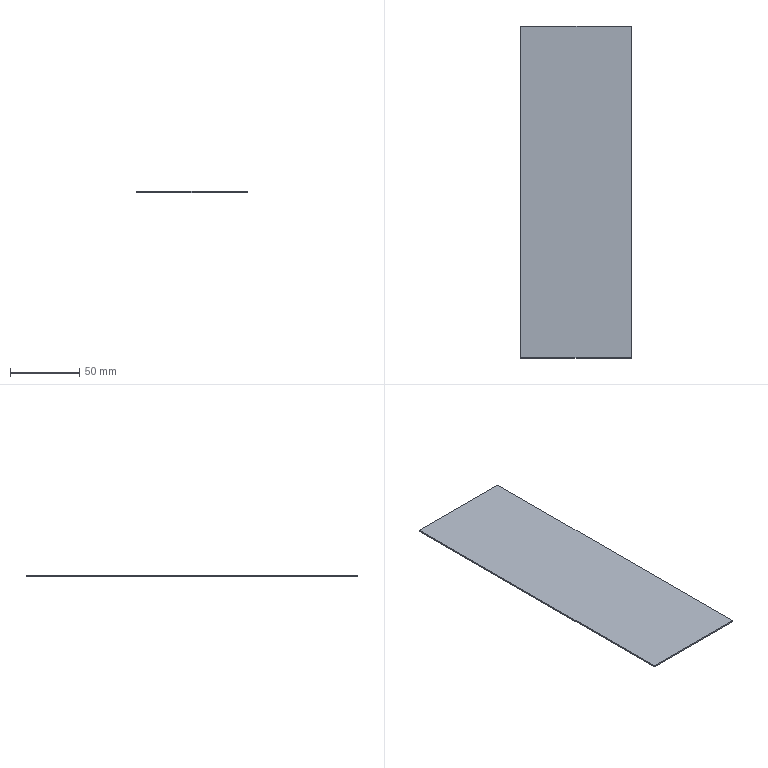Part | SolidWorks | features Extrusion 1 | 1 solid | 6 faces | box 80 x 240 x 1 mm | volume 19200 mm3 | plane 6
STEP:
#1=CARTESIAN_POINT('',(40.,-120.,0.));
#2=VERTEX_POINT('',#1);
#3=CARTESIAN_POINT('',(40.,120.,0.));
#4=VERTEX_POINT('',#3);
#5=CARTESIAN_POINT('',(40.,120.,0.));
#6=DIRECTION('',(0.,1.,0.));
#7=VECTOR('',#6,1000.);
#8=LINE('',#5,#7);
#9=EDGE_CURVE('',#2,#4,#8,.T.);
#10=ORIENTED_EDGE('',*,*,#9,.T.);
#11=CARTESIAN_POINT('',(40.,120.,1.));
#12=VERTEX_POINT('',#11);
#13=CARTESIAN_POINT('',(40.,120.,1.));
#14=DIRECTION('',(0.,0.,-1.));
#15=VECTOR('',#14,1000.);
#16=LINE('',#13,#15);
#17=EDGE_CURVE('',#12,#4,#16,.T.);
#18=ORIENTED_EDGE('',*,*,#17,.F.);
#19=CARTESIAN_POINT('',(40.,-120.,1.));
#20=VERTEX_POINT('',#19);
#21=CARTESIAN_POINT('',(40.,120.,1.));
#22=DIRECTION('',(0.,1.,0.));
#23=VECTOR('',#22,1000.);
#24=LINE('',#21,#23);
#25=EDGE_CURVE('',#20,#12,#24,.T.);
#26=ORIENTED_EDGE('',*,*,#25,.F.);
#27=CARTESIAN_POINT('',(40.,-120.,1.));
#28=DIRECTION('',(0.,0.,-1.));
#29=VECTOR('',#28,1000.);
#30=LINE('',#27,#29);
#31=EDGE_CURVE('',#20,#2,#30,.T.);
#32=ORIENTED_EDGE('',*,*,#31,.T.);
#33=EDGE_LOOP('',(#10,#18,#26,#32));
#34=FACE_OUTER_BOUND('',#33,.T.);
#35=CARTESIAN_POINT('',(40.,120.,1.));
#36=DIRECTION('',(-1.,0.,0.));
#37=DIRECTION('',(0.,-1.,0.));
#38=AXIS2_PLACEMENT_3D('',#35,#36,#37);
#39=PLANE('',#38);
#40=ADVANCED_FACE('',(#34),#39,.F.);
#41=CARTESIAN_POINT('',(-40.,120.,0.));
#42=VERTEX_POINT('',#41);
#43=CARTESIAN_POINT('',(-40.,120.,0.));
#44=DIRECTION('',(-1.,0.,0.));
#45=VECTOR('',#44,1000.);
#46=LINE('',#43,#45);
#47=EDGE_CURVE('',#4,#42,#46,.T.);
#48=ORIENTED_EDGE('',*,*,#47,.T.);
#49=CARTESIAN_POINT('',(-40.,120.,1.));
#50=VERTEX_POINT('',#49);
#51=CARTESIAN_POINT('',(-40.,120.,1.));
#52=DIRECTION('',(0.,0.,-1.));
#53=VECTOR('',#52,1000.);
#54=LINE('',#51,#53);
#55=EDGE_CURVE('',#50,#42,#54,.T.);
#56=ORIENTED_EDGE('',*,*,#55,.F.);
#57=CARTESIAN_POINT('',(-40.,120.,1.));
#58=DIRECTION('',(-1.,0.,0.));
#59=VECTOR('',#58,1000.);
#60=LINE('',#57,#59);
#61=EDGE_CURVE('',#12,#50,#60,.T.);
#62=ORIENTED_EDGE('',*,*,#61,.F.);
#63=ORIENTED_EDGE('',*,*,#17,.T.);
#64=EDGE_LOOP('',(#48,#56,#62,#63));
#65=FACE_OUTER_BOUND('',#64,.T.);
#66=CARTESIAN_POINT('',(-40.,120.,1.));
#67=DIRECTION('',(0.,-1.,0.));
#68=DIRECTION('',(0.,0.,-1.));
#69=AXIS2_PLACEMENT_3D('',#66,#67,#68);
#70=PLANE('',#69);
#71=ADVANCED_FACE('',(#65),#70,.F.);
#72=CARTESIAN_POINT('',(-40.,-120.,0.));
#73=VERTEX_POINT('',#72);
#74=CARTESIAN_POINT('',(-40.,120.,0.));
#75=DIRECTION('',(0.,-1.,0.));
#76=VECTOR('',#75,1000.);
#77=LINE('',#74,#76);
#78=EDGE_CURVE('',#42,#73,#77,.T.);
#79=ORIENTED_EDGE('',*,*,#78,.T.);
#80=CARTESIAN_POINT('',(-40.,-120.,1.));
#81=VERTEX_POINT('',#80);
#82=CARTESIAN_POINT('',(-40.,-120.,1.));
#83=DIRECTION('',(0.,0.,-1.));
#84=VECTOR('',#83,1000.);
#85=LINE('',#82,#84);
#86=EDGE_CURVE('',#81,#73,#85,.T.);
#87=ORIENTED_EDGE('',*,*,#86,.F.);
#88=CARTESIAN_POINT('',(-40.,120.,1.));
#89=DIRECTION('',(0.,-1.,0.));
#90=VECTOR('',#89,1000.);
#91=LINE('',#88,#90);
#92=EDGE_CURVE('',#50,#81,#91,.T.);
#93=ORIENTED_EDGE('',*,*,#92,.F.);
#94=ORIENTED_EDGE('',*,*,#55,.T.);
#95=EDGE_LOOP('',(#79,#87,#93,#94));
#96=FACE_OUTER_BOUND('',#95,.T.);
#97=CARTESIAN_POINT('',(-40.,120.,1.));
#98=DIRECTION('',(1.,0.,0.));
#99=DIRECTION('',(0.,1.,0.));
#100=AXIS2_PLACEMENT_3D('',#97,#98,#99);
#101=PLANE('',#100);
#102=ADVANCED_FACE('',(#96),#101,.F.);
#103=CARTESIAN_POINT('',(-40.,-120.,0.));
#104=DIRECTION('',(1.,0.,0.));
#105=VECTOR('',#104,1000.);
#106=LINE('',#103,#105);
#107=EDGE_CURVE('',#73,#2,#106,.T.);
#108=ORIENTED_EDGE('',*,*,#107,.T.);
#109=ORIENTED_EDGE('',*,*,#31,.F.);
#110=CARTESIAN_POINT('',(-40.,-120.,1.));
#111=DIRECTION('',(1.,0.,0.));
#112=VECTOR('',#111,1000.);
#113=LINE('',#110,#112);
#114=EDGE_CURVE('',#81,#20,#113,.T.);
#115=ORIENTED_EDGE('',*,*,#114,.F.);
#116=ORIENTED_EDGE('',*,*,#86,.T.);
#117=EDGE_LOOP('',(#108,#109,#115,#116));
#118=FACE_OUTER_BOUND('',#117,.T.);
#119=CARTESIAN_POINT('',(-40.,-120.,1.));
#120=DIRECTION('',(0.,1.,0.));
#121=DIRECTION('',(0.,0.,1.));
#122=AXIS2_PLACEMENT_3D('',#119,#120,#121);
#123=PLANE('',#122);
#124=ADVANCED_FACE('',(#118),#123,.F.);
#125=ORIENTED_EDGE('',*,*,#25,.T.);
#126=ORIENTED_EDGE('',*,*,#61,.T.);
#127=ORIENTED_EDGE('',*,*,#92,.T.);
#128=ORIENTED_EDGE('',*,*,#114,.T.);
#129=EDGE_LOOP('',(#125,#126,#127,#128));
#130=FACE_OUTER_BOUND('',#129,.T.);
#131=CARTESIAN_POINT('',(0.,0.,1.));
#132=DIRECTION('',(0.,0.,1.));
#133=DIRECTION('',(1.,0.,0.));
#134=AXIS2_PLACEMENT_3D('',#131,#132,#133);
#135=PLANE('',#134);
#136=ADVANCED_FACE('',(#130),#135,.T.);
#137=ORIENTED_EDGE('',*,*,#9,.F.);
#138=ORIENTED_EDGE('',*,*,#107,.F.);
#139=ORIENTED_EDGE('',*,*,#78,.F.);
#140=ORIENTED_EDGE('',*,*,#47,.F.);
#141=EDGE_LOOP('',(#137,#138,#139,#140));
#142=FACE_OUTER_BOUND('',#141,.T.);
#143=CARTESIAN_POINT('',(0.,0.,0.));
#144=DIRECTION('',(0.,0.,1.));
#145=DIRECTION('',(1.,0.,0.));
#146=AXIS2_PLACEMENT_3D('',#143,#144,#145);
#147=PLANE('',#146);
#148=ADVANCED_FACE('',(#142),#147,.F.);
#149=CLOSED_SHELL('',(#40,#71,#102,#124,#136,#148));
#150=MANIFOLD_SOLID_BREP('',#149);
#151=CARTESIAN_POINT('',(0.,0.,0.));
#152=DIRECTION('',(0.,0.,1.));
#153=DIRECTION('',(1.,0.,0.));
#154=AXIS2_PLACEMENT_3D('',#151,#152,#153);
#155=(LENGTH_UNIT()NAMED_UNIT(*)SI_UNIT(.MILLI.,.METRE.));
#156=UNCERTAINTY_MEASURE_WITH_UNIT(LENGTH_MEASURE(0.00001),#155,'','');
#157=(NAMED_UNIT(*)PLANE_ANGLE_UNIT()SI_UNIT($,.RADIAN.));
#158=(NAMED_UNIT(*)SI_UNIT($,.STERADIAN.)SOLID_ANGLE_UNIT());
#159=(GEOMETRIC_REPRESENTATION_CONTEXT(3)GLOBAL_UNCERTAINTY_ASSIGNED_CONTEXT((#156))GLOBAL_UNIT_ASSIGNED_CONTEXT((#155,#157,#158))REPRESENTATION_CONTEXT('',''));
#160=ADVANCED_BREP_SHAPE_REPRESENTATION('',(#150,#154),#159);